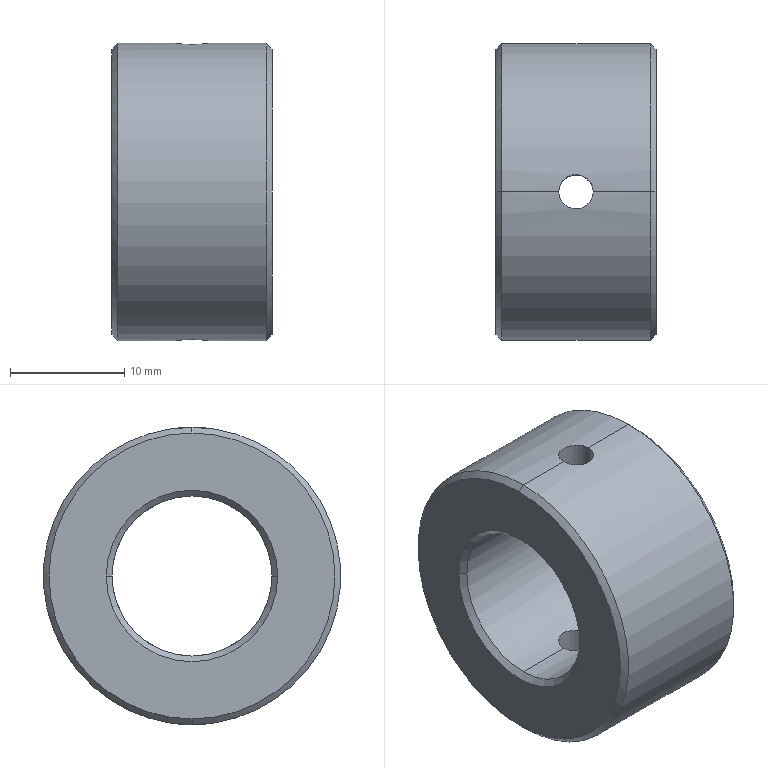Part | STEP file | mounting block_SUS304 | 1 solid | 18 faces | box 14 x 26 x 26 mm | volume 5161 mm3 | cylinder 8 | cone 8 | plane 2 | commonest cylinder face diameters 3 x4 14 x2 26 x2